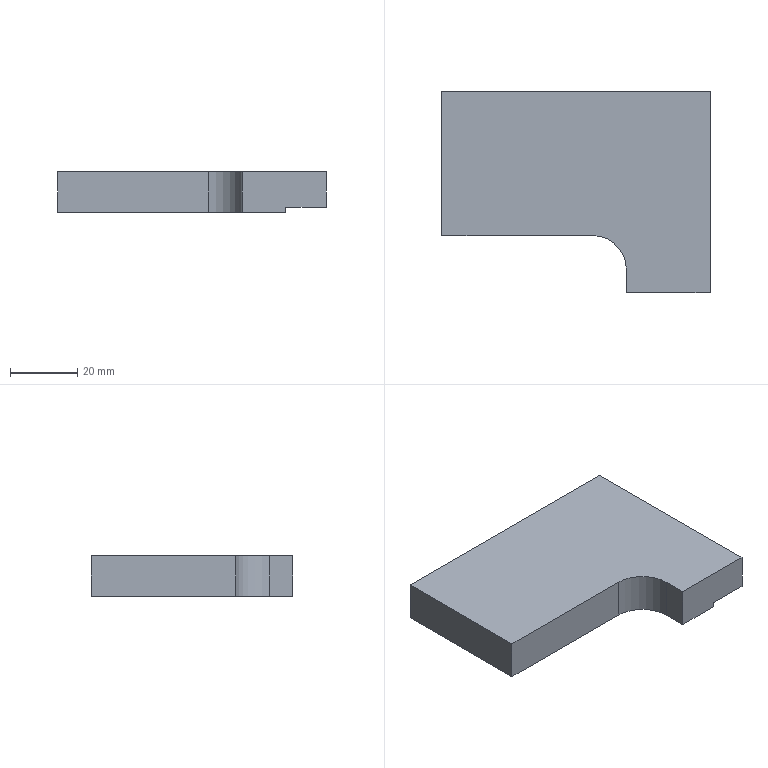Part | SolidWorks | features ICE 2, Extrusion 1, Fillet 1 | 1 solid | 11 faces | box 80 x 60 x 12 mm | volume 45558 mm3 | plane 10 | cylinder 1 | commonest cylinder face diameters 20 x1
STEP:
#1=CARTESIAN_POINT('',(40.,-30.,-4.5));
#2=VERTEX_POINT('',#1);
#3=CARTESIAN_POINT('',(40.,30.,-4.5));
#4=VERTEX_POINT('',#3);
#5=CARTESIAN_POINT('',(40.,30.,-4.5));
#6=DIRECTION('',(0.,1.,0.));
#7=VECTOR('',#6,1000.);
#8=LINE('',#5,#7);
#9=EDGE_CURVE('',#2,#4,#8,.T.);
#10=ORIENTED_EDGE('',*,*,#9,.T.);
#11=CARTESIAN_POINT('',(40.,30.,6.));
#12=VERTEX_POINT('',#11);
#13=CARTESIAN_POINT('',(40.,30.,6.));
#14=DIRECTION('',(0.,0.,-1.));
#15=VECTOR('',#14,1000.);
#16=LINE('',#13,#15);
#17=EDGE_CURVE('',#12,#4,#16,.T.);
#18=ORIENTED_EDGE('',*,*,#17,.F.);
#19=CARTESIAN_POINT('',(40.,-30.,6.));
#20=VERTEX_POINT('',#19);
#21=CARTESIAN_POINT('',(40.,-30.,6.));
#22=DIRECTION('',(0.,1.,0.));
#23=VECTOR('',#22,1000.);
#24=LINE('',#21,#23);
#25=EDGE_CURVE('',#20,#12,#24,.T.);
#26=ORIENTED_EDGE('',*,*,#25,.F.);
#27=CARTESIAN_POINT('',(40.,-30.,6.));
#28=DIRECTION('',(0.,0.,-1.));
#29=VECTOR('',#28,1000.);
#30=LINE('',#27,#29);
#31=EDGE_CURVE('',#20,#2,#30,.T.);
#32=ORIENTED_EDGE('',*,*,#31,.T.);
#33=EDGE_LOOP('',(#10,#18,#26,#32));
#34=FACE_OUTER_BOUND('',#33,.T.);
#35=CARTESIAN_POINT('',(40.,-30.,6.));
#36=DIRECTION('',(-1.,0.,0.));
#37=DIRECTION('',(0.,0.,1.));
#38=AXIS2_PLACEMENT_3D('',#35,#36,#37);
#39=PLANE('',#38);
#40=ADVANCED_FACE('',(#34),#39,.F.);
#41=CARTESIAN_POINT('',(28.,30.,-4.5));
#42=VERTEX_POINT('',#41);
#43=CARTESIAN_POINT('',(28.,30.,-6.));
#44=VERTEX_POINT('',#43);
#45=CARTESIAN_POINT('',(28.,30.,-4.5));
#46=DIRECTION('',(0.,0.,-1.));
#47=VECTOR('',#46,1000.);
#48=LINE('',#45,#47);
#49=EDGE_CURVE('',#42,#44,#48,.T.);
#50=ORIENTED_EDGE('',*,*,#49,.T.);
#51=CARTESIAN_POINT('',(-40.,30.,-6.));
#52=VERTEX_POINT('',#51);
#53=CARTESIAN_POINT('',(-40.,30.,-6.));
#54=DIRECTION('',(-1.,0.,0.));
#55=VECTOR('',#54,1000.);
#56=LINE('',#53,#55);
#57=EDGE_CURVE('',#44,#52,#56,.T.);
#58=ORIENTED_EDGE('',*,*,#57,.T.);
#59=CARTESIAN_POINT('',(-40.,30.,6.));
#60=VERTEX_POINT('',#59);
#61=CARTESIAN_POINT('',(-40.,30.,6.));
#62=DIRECTION('',(0.,0.,-1.));
#63=VECTOR('',#62,1000.);
#64=LINE('',#61,#63);
#65=EDGE_CURVE('',#60,#52,#64,.T.);
#66=ORIENTED_EDGE('',*,*,#65,.F.);
#67=CARTESIAN_POINT('',(-40.,30.,6.));
#68=DIRECTION('',(-1.,0.,0.));
#69=VECTOR('',#68,1000.);
#70=LINE('',#67,#69);
#71=EDGE_CURVE('',#12,#60,#70,.T.);
#72=ORIENTED_EDGE('',*,*,#71,.F.);
#73=ORIENTED_EDGE('',*,*,#17,.T.);
#74=CARTESIAN_POINT('',(40.,30.,-4.5));
#75=DIRECTION('',(-1.,0.,0.));
#76=VECTOR('',#75,1000.);
#77=LINE('',#74,#76);
#78=EDGE_CURVE('',#4,#42,#77,.T.);
#79=ORIENTED_EDGE('',*,*,#78,.T.);
#80=EDGE_LOOP('',(#50,#58,#66,#72,#73,#79));
#81=FACE_OUTER_BOUND('',#80,.T.);
#82=CARTESIAN_POINT('',(-40.,30.,6.));
#83=DIRECTION('',(0.,-1.,0.));
#84=DIRECTION('',(0.,0.,-1.));
#85=AXIS2_PLACEMENT_3D('',#82,#83,#84);
#86=PLANE('',#85);
#87=ADVANCED_FACE('',(#81),#86,.F.);
#88=CARTESIAN_POINT('',(15.,-30.,6.));
#89=VERTEX_POINT('',#88);
#90=CARTESIAN_POINT('',(-40.,-30.,6.));
#91=DIRECTION('',(1.,0.,0.));
#92=VECTOR('',#91,1000.);
#93=LINE('',#90,#92);
#94=EDGE_CURVE('',#89,#20,#93,.T.);
#95=ORIENTED_EDGE('',*,*,#94,.F.);
#96=CARTESIAN_POINT('',(15.,-30.,-6.));
#97=VERTEX_POINT('',#96);
#98=CARTESIAN_POINT('',(15.,-30.,6.001));
#99=DIRECTION('',(0.,0.,-1.));
#100=VECTOR('',#99,1000.);
#101=LINE('',#98,#100);
#102=EDGE_CURVE('',#89,#97,#101,.T.);
#103=ORIENTED_EDGE('',*,*,#102,.T.);
#104=CARTESIAN_POINT('',(28.,-30.,-6.));
#105=VERTEX_POINT('',#104);
#106=CARTESIAN_POINT('',(-40.,-30.,-6.));
#107=DIRECTION('',(1.,0.,0.));
#108=VECTOR('',#107,1000.);
#109=LINE('',#106,#108);
#110=EDGE_CURVE('',#97,#105,#109,.T.);
#111=ORIENTED_EDGE('',*,*,#110,.T.);
#112=CARTESIAN_POINT('',(28.,-30.,-4.5));
#113=VERTEX_POINT('',#112);
#114=CARTESIAN_POINT('',(28.,-30.,-4.5));
#115=DIRECTION('',(0.,0.,-1.));
#116=VECTOR('',#115,1000.);
#117=LINE('',#114,#116);
#118=EDGE_CURVE('',#113,#105,#117,.T.);
#119=ORIENTED_EDGE('',*,*,#118,.F.);
#120=CARTESIAN_POINT('',(40.,-30.,-4.5));
#121=DIRECTION('',(1.,0.,0.));
#122=VECTOR('',#121,1000.);
#123=LINE('',#120,#122);
#124=EDGE_CURVE('',#113,#2,#123,.T.);
#125=ORIENTED_EDGE('',*,*,#124,.T.);
#126=ORIENTED_EDGE('',*,*,#31,.F.);
#127=EDGE_LOOP('',(#95,#103,#111,#119,#125,#126));
#128=FACE_OUTER_BOUND('',#127,.T.);
#129=CARTESIAN_POINT('',(-40.,-30.,6.));
#130=DIRECTION('',(0.,1.,0.));
#131=DIRECTION('',(0.,0.,1.));
#132=AXIS2_PLACEMENT_3D('',#129,#130,#131);
#133=PLANE('',#132);
#134=ADVANCED_FACE('',(#128),#133,.F.);
#135=CARTESIAN_POINT('',(15.,-23.,-6.));
#136=VERTEX_POINT('',#135);
#137=CARTESIAN_POINT('',(15.,-30.,-6.));
#138=DIRECTION('',(0.,-1.,0.));
#139=VECTOR('',#138,1000.);
#140=LINE('',#137,#139);
#141=EDGE_CURVE('',#136,#97,#140,.T.);
#142=ORIENTED_EDGE('',*,*,#141,.F.);
#143=CARTESIAN_POINT('',(5.,-13.,-6.));
#144=VERTEX_POINT('',#143);
#145=CARTESIAN_POINT('',(5.,-23.,-6.));
#146=DIRECTION('',(0.,0.,1.));
#147=DIRECTION('',(-1.,0.,0.));
#148=AXIS2_PLACEMENT_3D('',#145,#146,#147);
#149=CIRCLE('',#148,10.);
#150=EDGE_CURVE('',#136,#144,#149,.T.);
#151=ORIENTED_EDGE('',*,*,#150,.T.);
#152=CARTESIAN_POINT('',(-40.,-13.,-6.));
#153=VERTEX_POINT('',#152);
#154=CARTESIAN_POINT('',(-40.,-13.,-6.));
#155=DIRECTION('',(1.,0.,0.));
#156=VECTOR('',#155,1000.);
#157=LINE('',#154,#156);
#158=EDGE_CURVE('',#153,#144,#157,.T.);
#159=ORIENTED_EDGE('',*,*,#158,.F.);
#160=CARTESIAN_POINT('',(-40.,-30.,-6.));
#161=DIRECTION('',(0.,-1.,0.));
#162=VECTOR('',#161,1000.);
#163=LINE('',#160,#162);
#164=EDGE_CURVE('',#52,#153,#163,.T.);
#165=ORIENTED_EDGE('',*,*,#164,.F.);
#166=ORIENTED_EDGE('',*,*,#57,.F.);
#167=CARTESIAN_POINT('',(28.,30.,-6.));
#168=DIRECTION('',(0.,-1.,0.));
#169=VECTOR('',#168,1000.);
#170=LINE('',#167,#169);
#171=EDGE_CURVE('',#44,#105,#170,.T.);
#172=ORIENTED_EDGE('',*,*,#171,.T.);
#173=ORIENTED_EDGE('',*,*,#110,.F.);
#174=EDGE_LOOP('',(#142,#151,#159,#165,#166,#172,#173));
#175=FACE_OUTER_BOUND('',#174,.T.);
#176=CARTESIAN_POINT('',(0.,0.,-6.));
#177=DIRECTION('',(0.,0.,-1.));
#178=DIRECTION('',(-1.,0.,0.));
#179=AXIS2_PLACEMENT_3D('',#176,#177,#178);
#180=PLANE('',#179);
#181=ADVANCED_FACE('',(#175),#180,.T.);
#182=ORIENTED_EDGE('',*,*,#164,.T.);
#183=CARTESIAN_POINT('',(-40.,-13.,6.));
#184=VERTEX_POINT('',#183);
#185=CARTESIAN_POINT('',(-40.,-13.,6.001));
#186=DIRECTION('',(0.,0.,-1.));
#187=VECTOR('',#186,1000.);
#188=LINE('',#185,#187);
#189=EDGE_CURVE('',#184,#153,#188,.T.);
#190=ORIENTED_EDGE('',*,*,#189,.F.);
#191=CARTESIAN_POINT('',(-40.,-30.,6.));
#192=DIRECTION('',(0.,-1.,0.));
#193=VECTOR('',#192,1000.);
#194=LINE('',#191,#193);
#195=EDGE_CURVE('',#60,#184,#194,.T.);
#196=ORIENTED_EDGE('',*,*,#195,.F.);
#197=ORIENTED_EDGE('',*,*,#65,.T.);
#198=EDGE_LOOP('',(#182,#190,#196,#197));
#199=FACE_OUTER_BOUND('',#198,.T.);
#200=CARTESIAN_POINT('',(-40.,-30.,6.));
#201=DIRECTION('',(1.,0.,0.));
#202=DIRECTION('',(0.,0.,-1.));
#203=AXIS2_PLACEMENT_3D('',#200,#201,#202);
#204=PLANE('',#203);
#205=ADVANCED_FACE('',(#199),#204,.F.);
#206=CARTESIAN_POINT('',(5.,-13.,6.));
#207=VERTEX_POINT('',#206);
#208=CARTESIAN_POINT('',(-40.,-13.,6.));
#209=DIRECTION('',(-1.,0.,0.));
#210=VECTOR('',#209,1000.);
#211=LINE('',#208,#210);
#212=EDGE_CURVE('',#207,#184,#211,.T.);
#213=ORIENTED_EDGE('',*,*,#212,.F.);
#214=CARTESIAN_POINT('',(15.,-23.,6.));
#215=VERTEX_POINT('',#214);
#216=CARTESIAN_POINT('',(5.,-23.,6.));
#217=DIRECTION('',(0.,0.,-1.));
#218=DIRECTION('',(-1.,0.,0.));
#219=AXIS2_PLACEMENT_3D('',#216,#217,#218);
#220=CIRCLE('',#219,10.);
#221=EDGE_CURVE('',#207,#215,#220,.T.);
#222=ORIENTED_EDGE('',*,*,#221,.T.);
#223=CARTESIAN_POINT('',(15.,-30.,6.));
#224=DIRECTION('',(0.,1.,0.));
#225=VECTOR('',#224,1000.);
#226=LINE('',#223,#225);
#227=EDGE_CURVE('',#89,#215,#226,.T.);
#228=ORIENTED_EDGE('',*,*,#227,.F.);
#229=ORIENTED_EDGE('',*,*,#94,.T.);
#230=ORIENTED_EDGE('',*,*,#25,.T.);
#231=ORIENTED_EDGE('',*,*,#71,.T.);
#232=ORIENTED_EDGE('',*,*,#195,.T.);
#233=EDGE_LOOP('',(#213,#222,#228,#229,#230,#231,#232));
#234=FACE_OUTER_BOUND('',#233,.T.);
#235=CARTESIAN_POINT('',(0.,0.,6.));
#236=DIRECTION('',(0.,0.,-1.));
#237=DIRECTION('',(-1.,0.,0.));
#238=AXIS2_PLACEMENT_3D('',#235,#236,#237);
#239=PLANE('',#238);
#240=ADVANCED_FACE('',(#234),#239,.F.);
#241=ORIENTED_EDGE('',*,*,#171,.F.);
#242=ORIENTED_EDGE('',*,*,#49,.F.);
#243=CARTESIAN_POINT('',(28.,30.,-4.5));
#244=DIRECTION('',(0.,-1.,0.));
#245=VECTOR('',#244,1000.);
#246=LINE('',#243,#245);
#247=EDGE_CURVE('',#42,#113,#246,.T.);
#248=ORIENTED_EDGE('',*,*,#247,.T.);
#249=ORIENTED_EDGE('',*,*,#118,.T.);
#250=EDGE_LOOP('',(#241,#242,#248,#249));
#251=FACE_OUTER_BOUND('',#250,.T.);
#252=CARTESIAN_POINT('',(28.,30.,-4.5));
#253=DIRECTION('',(1.,0.,0.));
#254=DIRECTION('',(0.,1.,0.));
#255=AXIS2_PLACEMENT_3D('',#252,#253,#254);
#256=PLANE('',#255);
#257=ADVANCED_FACE('',(#251),#256,.T.);
#258=ORIENTED_EDGE('',*,*,#9,.F.);
#259=ORIENTED_EDGE('',*,*,#124,.F.);
#260=ORIENTED_EDGE('',*,*,#247,.F.);
#261=ORIENTED_EDGE('',*,*,#78,.F.);
#262=EDGE_LOOP('',(#258,#259,#260,#261));
#263=FACE_OUTER_BOUND('',#262,.T.);
#264=CARTESIAN_POINT('',(0.,0.,-4.5));
#265=DIRECTION('',(0.,0.,-1.));
#266=DIRECTION('',(-1.,0.,0.));
#267=AXIS2_PLACEMENT_3D('',#264,#265,#266);
#268=PLANE('',#267);
#269=ADVANCED_FACE('',(#263),#268,.T.);
#270=ORIENTED_EDGE('',*,*,#227,.T.);
#271=CARTESIAN_POINT('',(15.,-23.,-6.));
#272=DIRECTION('',(0.,0.,-1.));
#273=VECTOR('',#272,1000.);
#274=LINE('',#271,#273);
#275=EDGE_CURVE('',#215,#136,#274,.T.);
#276=ORIENTED_EDGE('',*,*,#275,.T.);
#277=ORIENTED_EDGE('',*,*,#141,.T.);
#278=ORIENTED_EDGE('',*,*,#102,.F.);
#279=EDGE_LOOP('',(#270,#276,#277,#278));
#280=FACE_OUTER_BOUND('',#279,.T.);
#281=CARTESIAN_POINT('',(15.,-30.,6.001));
#282=DIRECTION('',(1.,0.,0.));
#283=DIRECTION('',(0.,0.,-1.));
#284=AXIS2_PLACEMENT_3D('',#281,#282,#283);
#285=PLANE('',#284);
#286=ADVANCED_FACE('',(#280),#285,.F.);
#287=ORIENTED_EDGE('',*,*,#158,.T.);
#288=CARTESIAN_POINT('',(5.,-13.,6.));
#289=DIRECTION('',(0.,0.,1.));
#290=VECTOR('',#289,1000.);
#291=LINE('',#288,#290);
#292=EDGE_CURVE('',#144,#207,#291,.T.);
#293=ORIENTED_EDGE('',*,*,#292,.T.);
#294=ORIENTED_EDGE('',*,*,#212,.T.);
#295=ORIENTED_EDGE('',*,*,#189,.T.);
#296=EDGE_LOOP('',(#287,#293,#294,#295));
#297=FACE_OUTER_BOUND('',#296,.T.);
#298=CARTESIAN_POINT('',(-40.,-13.,6.001));
#299=DIRECTION('',(0.,1.,0.));
#300=DIRECTION('',(-1.,0.,0.));
#301=AXIS2_PLACEMENT_3D('',#298,#299,#300);
#302=PLANE('',#301);
#303=ADVANCED_FACE('',(#297),#302,.F.);
#304=ORIENTED_EDGE('',*,*,#221,.F.);
#305=ORIENTED_EDGE('',*,*,#292,.F.);
#306=ORIENTED_EDGE('',*,*,#150,.F.);
#307=ORIENTED_EDGE('',*,*,#275,.F.);
#308=EDGE_LOOP('',(#304,#305,#306,#307));
#309=FACE_OUTER_BOUND('',#308,.T.);
#310=CARTESIAN_POINT('',(5.,-23.,6.001));
#311=DIRECTION('',(0.,0.,1.));
#312=DIRECTION('',(1.,0.,0.));
#313=AXIS2_PLACEMENT_3D('',#310,#311,#312);
#314=CYLINDRICAL_SURFACE('',#313,10.);
#315=ADVANCED_FACE('',(#309),#314,.F.);
#316=CLOSED_SHELL('',(#40,#87,#134,#181,#205,#240,#257,#269,#286,#303,#315));
#317=MANIFOLD_SOLID_BREP('',#316);
#318=CARTESIAN_POINT('',(0.,0.,0.));
#319=DIRECTION('',(0.,0.,1.));
#320=DIRECTION('',(1.,0.,0.));
#321=AXIS2_PLACEMENT_3D('',#318,#319,#320);
#322=(LENGTH_UNIT()NAMED_UNIT(*)SI_UNIT(.MILLI.,.METRE.));
#323=UNCERTAINTY_MEASURE_WITH_UNIT(LENGTH_MEASURE(0.00001),#322,'','');
#324=(NAMED_UNIT(*)PLANE_ANGLE_UNIT()SI_UNIT($,.RADIAN.));
#325=(NAMED_UNIT(*)SI_UNIT($,.STERADIAN.)SOLID_ANGLE_UNIT());
#326=(GEOMETRIC_REPRESENTATION_CONTEXT(3)GLOBAL_UNCERTAINTY_ASSIGNED_CONTEXT((#323))GLOBAL_UNIT_ASSIGNED_CONTEXT((#322,#324,#325))REPRESENTATION_CONTEXT('',''));
#327=ADVANCED_BREP_SHAPE_REPRESENTATION('',(#317,#321),#326);